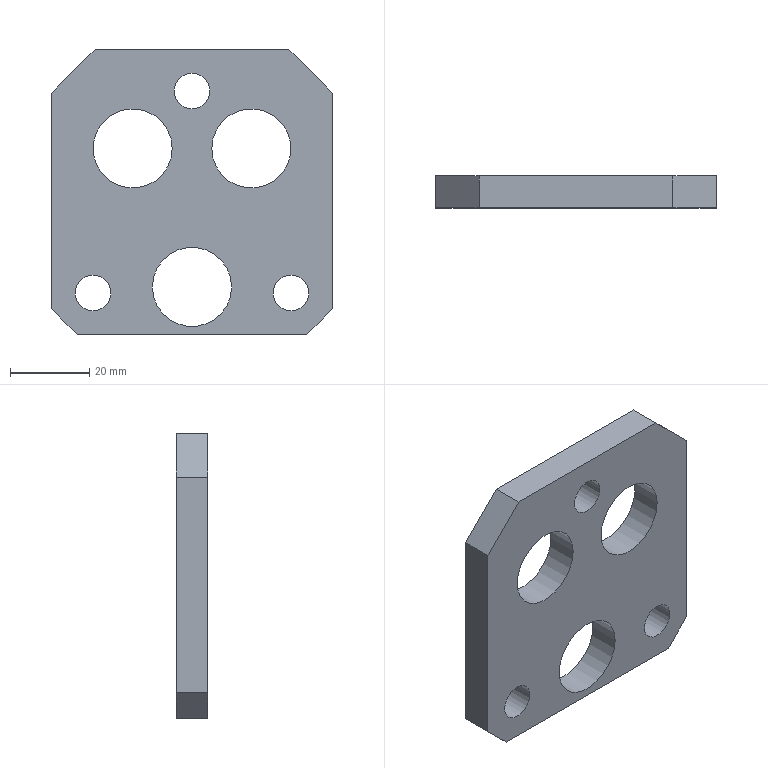Part | STEP file | 1_id610_x_t | 1 solid | 16 faces | box 71 x 8 x 72 mm | volume 30523 mm3 | plane 10 | cylinder 6 | commonest cylinder face diameters 9 x3 20 x3
STEP:
#1=CARTESIAN_POINT('',(0.,0.,0.));
#2=DIRECTION('',(0.,0.,1.));
#3=DIRECTION('',(1.,0.,0.));
#4=AXIS2_PLACEMENT_3D('',#1,#2,#3);
#5=CARTESIAN_POINT('',(720.425,281.527,-85.684));
#6=VERTEX_POINT('',#5);
#7=CARTESIAN_POINT('',(724.925,281.527,-85.684));
#8=DIRECTION('',(0.,1.,0.));
#9=DIRECTION('',(-1.,0.,0.));
#10=AXIS2_PLACEMENT_3D('',#7,#8,#9);
#11=CIRCLE('',#10,4.5);
#12=CARTESIAN_POINT('',(724.925,289.527,-85.684));
#13=DIRECTION('',(0.,-1.,0.));
#14=DIRECTION('',(-1.,0.,0.));
#15=AXIS2_PLACEMENT_3D('',#12,#13,#14);
#16=CYLINDRICAL_SURFACE('',#15,4.5);
#17=CARTESIAN_POINT('',(6.283,8.));
#18=DIRECTION('',(-1.,0.));
#19=VECTOR('',#18,1.);
#20=LINE('',#17,#19);
#21=(GEOMETRIC_REPRESENTATION_CONTEXT(2)PARAMETRIC_REPRESENTATION_CONTEXT()REPRESENTATION_CONTEXT('',''));
#22=DEFINITIONAL_REPRESENTATION('',(#20),#21);
#23=PCURVE('',#16,#22);
#24=CARTESIAN_POINT('',(699.125,281.527,-9.148));
#25=DIRECTION('',(0.,1.,0.));
#26=DIRECTION('',(1.,0.,0.));
#27=AXIS2_PLACEMENT_3D('',#24,#25,#26);
#28=PLANE('',#27);
#29=CARTESIAN_POINT('',(25.8,76.536));
#30=DIRECTION('',(-1.,0.));
#31=AXIS2_PLACEMENT_2D('',#29,#30);
#32=CIRCLE('',#31,4.5);
#33=(GEOMETRIC_REPRESENTATION_CONTEXT(2)PARAMETRIC_REPRESENTATION_CONTEXT()REPRESENTATION_CONTEXT('',''));
#34=DEFINITIONAL_REPRESENTATION('',(#32),#33);
#35=PCURVE('',#28,#34);
#36=SURFACE_CURVE('',#11,(#23,#35),.PCURVE_S1.);
#37=EDGE_CURVE('',#6,#6,#36,.T.);
#38=ORIENTED_EDGE('',*,*,#37,.T.);
#39=CARTESIAN_POINT('',(720.425,289.527,-85.684));
#40=VERTEX_POINT('',#39);
#41=CARTESIAN_POINT('',(720.425,289.527,-85.684));
#42=CARTESIAN_POINT('',(720.425,281.527,-85.684));
#43=B_SPLINE_CURVE_WITH_KNOTS('',1,(#41,#42),.UNSPECIFIED.,.F.,.F.,(2,2),(0.,8.),.PIECEWISE_BEZIER_KNOTS.);
#44=CARTESIAN_POINT('',(0.,0.));
#45=DIRECTION('',(0.,1.));
#46=VECTOR('',#45,1.);
#47=LINE('',#44,#46);
#48=(GEOMETRIC_REPRESENTATION_CONTEXT(2)PARAMETRIC_REPRESENTATION_CONTEXT()REPRESENTATION_CONTEXT('',''));
#49=DEFINITIONAL_REPRESENTATION('',(#47),#48);
#50=PCURVE('',#16,#49);
#51=CARTESIAN_POINT('',(6.283,0.));
#52=DIRECTION('',(0.,1.));
#53=VECTOR('',#52,1.);
#54=LINE('',#51,#53);
#55=(GEOMETRIC_REPRESENTATION_CONTEXT(2)PARAMETRIC_REPRESENTATION_CONTEXT()REPRESENTATION_CONTEXT('',''));
#56=DEFINITIONAL_REPRESENTATION('',(#54),#55);
#57=PCURVE('',#16,#56);
#58=SEAM_CURVE('',#43,(#50,#57),.PCURVE_S1.);
#59=EDGE_CURVE('',#40,#6,#58,.T.);
#60=ORIENTED_EDGE('',*,*,#59,.F.);
#61=CARTESIAN_POINT('',(729.425,289.527,-85.684));
#62=VERTEX_POINT('',#61);
#63=CARTESIAN_POINT('',(724.925,289.527,-85.684));
#64=DIRECTION('',(0.,-1.,0.));
#65=DIRECTION('',(1.,0.,0.));
#66=AXIS2_PLACEMENT_3D('',#63,#64,#65);
#67=CIRCLE('',#66,4.5);
#68=CARTESIAN_POINT('',(-3.142,0.));
#69=DIRECTION('',(1.,0.));
#70=VECTOR('',#69,1.);
#71=LINE('',#68,#70);
#72=(GEOMETRIC_REPRESENTATION_CONTEXT(2)PARAMETRIC_REPRESENTATION_CONTEXT()REPRESENTATION_CONTEXT('',''));
#73=DEFINITIONAL_REPRESENTATION('',(#71),#72);
#74=PCURVE('',#16,#73);
#75=CARTESIAN_POINT('',(699.125,289.527,-9.148));
#76=DIRECTION('',(0.,1.,0.));
#77=DIRECTION('',(1.,0.,0.));
#78=AXIS2_PLACEMENT_3D('',#75,#76,#77);
#79=PLANE('',#78);
#80=CARTESIAN_POINT('',(30.3,76.536));
#81=CARTESIAN_POINT('',(30.3,68.742));
#82=CARTESIAN_POINT('',(23.55,72.639));
#83=CARTESIAN_POINT('',(16.8,76.536));
#84=CARTESIAN_POINT('',(23.55,80.433));
#85=CARTESIAN_POINT('',(30.3,84.33));
#86=CARTESIAN_POINT('',(30.3,76.536));
#87=(BOUNDED_CURVE()B_SPLINE_CURVE(2,(#80,#81,#82,#83,#84,#85,#86),.UNSPECIFIED.,.T.,.F.)B_SPLINE_CURVE_WITH_KNOTS((1,2,2,2,2,1),(-2.094,0.,2.094,4.189,6.283,8.378),.UNSPECIFIED.)CURVE()GEOMETRIC_REPRESENTATION_ITEM()RATIONAL_B_SPLINE_CURVE((1.,0.5,1.,0.5,1.,0.5,1.))REPRESENTATION_ITEM(''));
#88=(GEOMETRIC_REPRESENTATION_CONTEXT(2)PARAMETRIC_REPRESENTATION_CONTEXT()REPRESENTATION_CONTEXT('',''));
#89=DEFINITIONAL_REPRESENTATION('',(#87),#88);
#90=PCURVE('',#79,#89);
#91=SURFACE_CURVE('',#67,(#74,#90),.PCURVE_S1.);
#92=EDGE_CURVE('',#40,#62,#91,.T.);
#93=ORIENTED_EDGE('',*,*,#92,.T.);
#94=CARTESIAN_POINT('',(724.925,289.527,-85.684));
#95=DIRECTION('',(0.,-1.,0.));
#96=DIRECTION('',(1.,0.,0.));
#97=AXIS2_PLACEMENT_3D('',#94,#95,#96);
#98=CIRCLE('',#97,4.5);
#99=CARTESIAN_POINT('',(3.142,0.));
#100=DIRECTION('',(1.,0.));
#101=VECTOR('',#100,1.);
#102=LINE('',#99,#101);
#103=(GEOMETRIC_REPRESENTATION_CONTEXT(2)PARAMETRIC_REPRESENTATION_CONTEXT()REPRESENTATION_CONTEXT('',''));
#104=DEFINITIONAL_REPRESENTATION('',(#102),#103);
#105=PCURVE('',#16,#104);
#106=CARTESIAN_POINT('',(30.3,76.536));
#107=CARTESIAN_POINT('',(30.3,68.742));
#108=CARTESIAN_POINT('',(23.55,72.639));
#109=CARTESIAN_POINT('',(16.8,76.536));
#110=CARTESIAN_POINT('',(23.55,80.433));
#111=CARTESIAN_POINT('',(30.3,84.33));
#112=CARTESIAN_POINT('',(30.3,76.536));
#113=(BOUNDED_CURVE()B_SPLINE_CURVE(2,(#106,#107,#108,#109,#110,#111,#112),.UNSPECIFIED.,.T.,.F.)B_SPLINE_CURVE_WITH_KNOTS((1,2,2,2,2,1),(-2.094,0.,2.094,4.189,6.283,8.378),.UNSPECIFIED.)CURVE()GEOMETRIC_REPRESENTATION_ITEM()RATIONAL_B_SPLINE_CURVE((1.,0.5,1.,0.5,1.,0.5,1.))REPRESENTATION_ITEM(''));
#114=(GEOMETRIC_REPRESENTATION_CONTEXT(2)PARAMETRIC_REPRESENTATION_CONTEXT()REPRESENTATION_CONTEXT('',''));
#115=DEFINITIONAL_REPRESENTATION('',(#113),#114);
#116=PCURVE('',#79,#115);
#117=SURFACE_CURVE('',#98,(#105,#116),.PCURVE_S1.);
#118=EDGE_CURVE('',#62,#40,#117,.T.);
#119=ORIENTED_EDGE('',*,*,#118,.T.);
#120=ORIENTED_EDGE('',*,*,#59,.T.);
#121=EDGE_LOOP('',(#38,#60,#93,#119,#120));
#122=FACE_BOUND('',#121,.F.);
#123=ADVANCED_FACE('',(#122),#16,.F.);
#124=CARTESIAN_POINT('',(774.425,289.527,-24.184));
#125=VERTEX_POINT('',#124);
#126=CARTESIAN_POINT('',(785.425,289.527,-35.184));
#127=VERTEX_POINT('',#126);
#128=CARTESIAN_POINT('',(774.425,289.527,-24.184));
#129=DIRECTION('',(0.7071,0.,-0.7071));
#130=VECTOR('',#129,1.);
#131=LINE('',#128,#130);
#132=CARTESIAN_POINT('',(75.3,15.036));
#133=DIRECTION('',(0.7071,0.7071));
#134=VECTOR('',#133,1.);
#135=LINE('',#132,#134);
#136=(GEOMETRIC_REPRESENTATION_CONTEXT(2)PARAMETRIC_REPRESENTATION_CONTEXT()REPRESENTATION_CONTEXT('',''));
#137=DEFINITIONAL_REPRESENTATION('',(#135),#136);
#138=PCURVE('',#79,#137);
#139=CARTESIAN_POINT('',(729.257,289.527,20.984));
#140=DIRECTION('',(-0.7071,0.,-0.7071));
#141=DIRECTION('',(-0.7071,0.,0.7071));
#142=AXIS2_PLACEMENT_3D('',#139,#140,#141);
#143=PLANE('',#142);
#144=CARTESIAN_POINT('',(-63.877,0.));
#145=DIRECTION('',(-1.,0.));
#146=VECTOR('',#145,1.);
#147=LINE('',#144,#146);
#148=(GEOMETRIC_REPRESENTATION_CONTEXT(2)PARAMETRIC_REPRESENTATION_CONTEXT()REPRESENTATION_CONTEXT('',''));
#149=DEFINITIONAL_REPRESENTATION('',(#147),#148);
#150=PCURVE('',#143,#149);
#151=SURFACE_CURVE('',#131,(#138,#150),.PCURVE_S1.);
#152=EDGE_CURVE('',#125,#127,#151,.T.);
#153=ORIENTED_EDGE('',*,*,#152,.T.);
#154=CARTESIAN_POINT('',(785.425,289.527,-89.684));
#155=VERTEX_POINT('',#154);
#156=CARTESIAN_POINT('',(785.425,289.527,-35.184));
#157=DIRECTION('',(0.,0.,-1.));
#158=VECTOR('',#157,1.);
#159=LINE('',#156,#158);
#160=CARTESIAN_POINT('',(86.3,26.036));
#161=DIRECTION('',(0.,1.));
#162=VECTOR('',#161,1.);
#163=LINE('',#160,#162);
#164=(GEOMETRIC_REPRESENTATION_CONTEXT(2)PARAMETRIC_REPRESENTATION_CONTEXT()REPRESENTATION_CONTEXT('',''));
#165=DEFINITIONAL_REPRESENTATION('',(#163),#164);
#166=PCURVE('',#79,#165);
#167=CARTESIAN_POINT('',(785.425,289.527,159.705));
#168=DIRECTION('',(-1.,0.,0.));
#169=DIRECTION('',(0.,1.,0.));
#170=AXIS2_PLACEMENT_3D('',#167,#168,#169);
#171=PLANE('',#170);
#172=CARTESIAN_POINT('',(0.,194.889));
#173=DIRECTION('',(0.,1.));
#174=VECTOR('',#173,1.);
#175=LINE('',#172,#174);
#176=(GEOMETRIC_REPRESENTATION_CONTEXT(2)PARAMETRIC_REPRESENTATION_CONTEXT()REPRESENTATION_CONTEXT('',''));
#177=DEFINITIONAL_REPRESENTATION('',(#175),#176);
#178=PCURVE('',#171,#177);
#179=SURFACE_CURVE('',#159,(#166,#178),.PCURVE_S1.);
#180=EDGE_CURVE('',#127,#155,#179,.T.);
#181=ORIENTED_EDGE('',*,*,#180,.T.);
#182=CARTESIAN_POINT('',(778.925,289.527,-96.184));
#183=VERTEX_POINT('',#182);
#184=CARTESIAN_POINT('',(785.425,289.527,-89.684));
#185=DIRECTION('',(-0.7071,0.,-0.7071));
#186=VECTOR('',#185,1.);
#187=LINE('',#184,#186);
#188=CARTESIAN_POINT('',(86.3,80.536));
#189=DIRECTION('',(-0.7071,0.7071));
#190=VECTOR('',#189,1.);
#191=LINE('',#188,#190);
#192=(GEOMETRIC_REPRESENTATION_CONTEXT(2)PARAMETRIC_REPRESENTATION_CONTEXT()REPRESENTATION_CONTEXT('',''));
#193=DEFINITIONAL_REPRESENTATION('',(#191),#192);
#194=PCURVE('',#79,#193);
#195=CARTESIAN_POINT('',(775.043,289.527,-100.066));
#196=DIRECTION('',(-0.7071,0.,0.7071));
#197=DIRECTION('',(0.7071,0.,0.7071));
#198=AXIS2_PLACEMENT_3D('',#195,#196,#197);
#199=PLANE('',#198);
#200=CARTESIAN_POINT('',(14.682,0.));
#201=DIRECTION('',(-1.,0.));
#202=VECTOR('',#201,1.);
#203=LINE('',#200,#202);
#204=(GEOMETRIC_REPRESENTATION_CONTEXT(2)PARAMETRIC_REPRESENTATION_CONTEXT()REPRESENTATION_CONTEXT('',''));
#205=DEFINITIONAL_REPRESENTATION('',(#203),#204);
#206=PCURVE('',#199,#205);
#207=SURFACE_CURVE('',#187,(#194,#206),.PCURVE_S1.);
#208=EDGE_CURVE('',#155,#183,#207,.T.);
#209=ORIENTED_EDGE('',*,*,#208,.T.);
#210=CARTESIAN_POINT('',(720.925,289.527,-96.184));
#211=VERTEX_POINT('',#210);
#212=CARTESIAN_POINT('',(778.925,289.527,-96.184));
#213=DIRECTION('',(-1.,0.,0.));
#214=VECTOR('',#213,1.);
#215=LINE('',#212,#214);
#216=CARTESIAN_POINT('',(79.8,87.036));
#217=DIRECTION('',(-1.,0.));
#218=VECTOR('',#217,1.);
#219=LINE('',#216,#218);
#220=(GEOMETRIC_REPRESENTATION_CONTEXT(2)PARAMETRIC_REPRESENTATION_CONTEXT()REPRESENTATION_CONTEXT('',''));
#221=DEFINITIONAL_REPRESENTATION('',(#219),#220);
#222=PCURVE('',#79,#221);
#223=CARTESIAN_POINT('',(699.125,289.527,-96.184));
#224=DIRECTION('',(0.,0.,1.));
#225=DIRECTION('',(0.,-1.,0.));
#226=AXIS2_PLACEMENT_3D('',#223,#224,#225);
#227=PLANE('',#226);
#228=CARTESIAN_POINT('',(0.,79.8));
#229=DIRECTION('',(0.,-1.));
#230=VECTOR('',#229,1.);
#231=LINE('',#228,#230);
#232=(GEOMETRIC_REPRESENTATION_CONTEXT(2)PARAMETRIC_REPRESENTATION_CONTEXT()REPRESENTATION_CONTEXT('',''));
#233=DEFINITIONAL_REPRESENTATION('',(#231),#232);
#234=PCURVE('',#227,#233);
#235=SURFACE_CURVE('',#215,(#222,#234),.PCURVE_S1.);
#236=EDGE_CURVE('',#183,#211,#235,.T.);
#237=ORIENTED_EDGE('',*,*,#236,.T.);
#238=CARTESIAN_POINT('',(714.425,289.527,-89.684));
#239=VERTEX_POINT('',#238);
#240=CARTESIAN_POINT('',(720.925,289.527,-96.184));
#241=DIRECTION('',(-0.7071,0.,0.7071));
#242=VECTOR('',#241,1.);
#243=LINE('',#240,#242);
#244=CARTESIAN_POINT('',(21.8,87.036));
#245=DIRECTION('',(-0.7071,-0.7071));
#246=VECTOR('',#245,1.);
#247=LINE('',#244,#246);
#248=(GEOMETRIC_REPRESENTATION_CONTEXT(2)PARAMETRIC_REPRESENTATION_CONTEXT()REPRESENTATION_CONTEXT('',''));
#249=DEFINITIONAL_REPRESENTATION('',(#247),#248);
#250=PCURVE('',#79,#249);
#251=CARTESIAN_POINT('',(674.007,289.527,-49.266));
#252=DIRECTION('',(0.7071,0.,0.7071));
#253=DIRECTION('',(0.7071,0.,-0.7071));
#254=AXIS2_PLACEMENT_3D('',#251,#252,#253);
#255=PLANE('',#254);
#256=CARTESIAN_POINT('',(66.352,0.));
#257=DIRECTION('',(-1.,0.));
#258=VECTOR('',#257,1.);
#259=LINE('',#256,#258);
#260=(GEOMETRIC_REPRESENTATION_CONTEXT(2)PARAMETRIC_REPRESENTATION_CONTEXT()REPRESENTATION_CONTEXT('',''));
#261=DEFINITIONAL_REPRESENTATION('',(#259),#260);
#262=PCURVE('',#255,#261);
#263=SURFACE_CURVE('',#243,(#250,#262),.PCURVE_S1.);
#264=EDGE_CURVE('',#211,#239,#263,.T.);
#265=ORIENTED_EDGE('',*,*,#264,.T.);
#266=CARTESIAN_POINT('',(714.425,289.527,-35.184));
#267=VERTEX_POINT('',#266);
#268=CARTESIAN_POINT('',(714.425,289.527,-89.684));
#269=DIRECTION('',(0.,0.,1.));
#270=VECTOR('',#269,1.);
#271=LINE('',#268,#270);
#272=CARTESIAN_POINT('',(15.3,80.536));
#273=DIRECTION('',(0.,-1.));
#274=VECTOR('',#273,1.);
#275=LINE('',#272,#274);
#276=(GEOMETRIC_REPRESENTATION_CONTEXT(2)PARAMETRIC_REPRESENTATION_CONTEXT()REPRESENTATION_CONTEXT('',''));
#277=DEFINITIONAL_REPRESENTATION('',(#275),#276);
#278=PCURVE('',#79,#277);
#279=CARTESIAN_POINT('',(714.425,289.527,-255.215));
#280=DIRECTION('',(1.,0.,0.));
#281=DIRECTION('',(0.,-1.,0.));
#282=AXIS2_PLACEMENT_3D('',#279,#280,#281);
#283=PLANE('',#282);
#284=CARTESIAN_POINT('',(0.,-165.531));
#285=DIRECTION('',(0.,-1.));
#286=VECTOR('',#285,1.);
#287=LINE('',#284,#286);
#288=(GEOMETRIC_REPRESENTATION_CONTEXT(2)PARAMETRIC_REPRESENTATION_CONTEXT()REPRESENTATION_CONTEXT('',''));
#289=DEFINITIONAL_REPRESENTATION('',(#287),#288);
#290=PCURVE('',#283,#289);
#291=SURFACE_CURVE('',#271,(#278,#290),.PCURVE_S1.);
#292=EDGE_CURVE('',#239,#267,#291,.T.);
#293=ORIENTED_EDGE('',*,*,#292,.T.);
#294=CARTESIAN_POINT('',(725.425,289.527,-24.184));
#295=VERTEX_POINT('',#294);
#296=CARTESIAN_POINT('',(714.425,289.527,-35.184));
#297=DIRECTION('',(0.7071,0.,0.7071));
#298=VECTOR('',#297,1.);
#299=LINE('',#296,#298);
#300=CARTESIAN_POINT('',(15.3,26.036));
#301=DIRECTION('',(0.7071,-0.7071));
#302=VECTOR('',#301,1.);
#303=LINE('',#300,#302);
#304=(GEOMETRIC_REPRESENTATION_CONTEXT(2)PARAMETRIC_REPRESENTATION_CONTEXT()REPRESENTATION_CONTEXT('',''));
#305=DEFINITIONAL_REPRESENTATION('',(#303),#304);
#306=PCURVE('',#79,#305);
#307=CARTESIAN_POINT('',(719.793,289.527,-29.816));
#308=DIRECTION('',(0.7071,0.,-0.7071));
#309=DIRECTION('',(-0.7071,0.,-0.7071));
#310=AXIS2_PLACEMENT_3D('',#307,#308,#309);
#311=PLANE('',#310);
#312=CARTESIAN_POINT('',(7.591,0.));
#313=DIRECTION('',(-1.,0.));
#314=VECTOR('',#313,1.);
#315=LINE('',#312,#314);
#316=(GEOMETRIC_REPRESENTATION_CONTEXT(2)PARAMETRIC_REPRESENTATION_CONTEXT()REPRESENTATION_CONTEXT('',''));
#317=DEFINITIONAL_REPRESENTATION('',(#315),#316);
#318=PCURVE('',#311,#317);
#319=SURFACE_CURVE('',#299,(#306,#318),.PCURVE_S1.);
#320=EDGE_CURVE('',#267,#295,#319,.T.);
#321=ORIENTED_EDGE('',*,*,#320,.T.);
#322=CARTESIAN_POINT('',(725.425,289.527,-24.184));
#323=DIRECTION('',(1.,0.,0.));
#324=VECTOR('',#323,1.);
#325=LINE('',#322,#324);
#326=CARTESIAN_POINT('',(26.3,15.036));
#327=DIRECTION('',(1.,0.));
#328=VECTOR('',#327,1.);
#329=LINE('',#326,#328);
#330=(GEOMETRIC_REPRESENTATION_CONTEXT(2)PARAMETRIC_REPRESENTATION_CONTEXT()REPRESENTATION_CONTEXT('',''));
#331=DEFINITIONAL_REPRESENTATION('',(#329),#330);
#332=PCURVE('',#79,#331);
#333=CARTESIAN_POINT('',(699.125,289.527,-24.184));
#334=DIRECTION('',(0.,0.,-1.));
#335=DIRECTION('',(0.,1.,0.));
#336=AXIS2_PLACEMENT_3D('',#333,#334,#335);
#337=PLANE('',#336);
#338=CARTESIAN_POINT('',(0.,26.3));
#339=DIRECTION('',(0.,1.));
#340=VECTOR('',#339,1.);
#341=LINE('',#338,#340);
#342=(GEOMETRIC_REPRESENTATION_CONTEXT(2)PARAMETRIC_REPRESENTATION_CONTEXT()REPRESENTATION_CONTEXT('',''));
#343=DEFINITIONAL_REPRESENTATION('',(#341),#342);
#344=PCURVE('',#337,#343);
#345=SURFACE_CURVE('',#325,(#332,#344),.PCURVE_S1.);
#346=EDGE_CURVE('',#295,#125,#345,.T.);
#347=ORIENTED_EDGE('',*,*,#346,.T.);
#348=EDGE_LOOP('',(#153,#181,#209,#237,#265,#293,#321,#347));
#349=FACE_BOUND('',#348,.T.);
#350=CARTESIAN_POINT('',(774.925,289.527,-49.184));
#351=VERTEX_POINT('',#350);
#352=CARTESIAN_POINT('',(754.925,289.527,-49.184));
#353=VERTEX_POINT('',#352);
#354=CARTESIAN_POINT('',(764.925,289.527,-49.184));
#355=DIRECTION('',(0.,-1.,0.));
#356=DIRECTION('',(1.,0.,0.));
#357=AXIS2_PLACEMENT_3D('',#354,#355,#356);
#358=CIRCLE('',#357,10.);
#359=CARTESIAN_POINT('',(75.8,40.036));
#360=CARTESIAN_POINT('',(75.8,22.715));
#361=CARTESIAN_POINT('',(60.8,31.376));
#362=CARTESIAN_POINT('',(45.8,40.036));
#363=CARTESIAN_POINT('',(60.8,48.696));
#364=CARTESIAN_POINT('',(75.8,57.357));
#365=CARTESIAN_POINT('',(75.8,40.036));
#366=(BOUNDED_CURVE()B_SPLINE_CURVE(2,(#359,#360,#361,#362,#363,#364,#365),.UNSPECIFIED.,.T.,.F.)B_SPLINE_CURVE_WITH_KNOTS((1,2,2,2,2,1),(-2.094,0.,2.094,4.189,6.283,8.378),.UNSPECIFIED.)CURVE()GEOMETRIC_REPRESENTATION_ITEM()RATIONAL_B_SPLINE_CURVE((1.,0.5,1.,0.5,1.,0.5,1.))REPRESENTATION_ITEM(''));
#367=(GEOMETRIC_REPRESENTATION_CONTEXT(2)PARAMETRIC_REPRESENTATION_CONTEXT()REPRESENTATION_CONTEXT('',''));
#368=DEFINITIONAL_REPRESENTATION('',(#366),#367);
#369=PCURVE('',#79,#368);
#370=CARTESIAN_POINT('',(764.925,289.527,-49.184));
#371=DIRECTION('',(0.,-1.,0.));
#372=DIRECTION('',(-1.,0.,0.));
#373=AXIS2_PLACEMENT_3D('',#370,#371,#372);
#374=CYLINDRICAL_SURFACE('',#373,10.);
#375=CARTESIAN_POINT('',(3.142,0.));
#376=DIRECTION('',(1.,0.));
#377=VECTOR('',#376,1.);
#378=LINE('',#375,#377);
#379=(GEOMETRIC_REPRESENTATION_CONTEXT(2)PARAMETRIC_REPRESENTATION_CONTEXT()REPRESENTATION_CONTEXT('',''));
#380=DEFINITIONAL_REPRESENTATION('',(#378),#379);
#381=PCURVE('',#374,#380);
#382=SURFACE_CURVE('',#358,(#369,#381),.PCURVE_S1.);
#383=EDGE_CURVE('',#351,#353,#382,.T.);
#384=ORIENTED_EDGE('',*,*,#383,.T.);
#385=CARTESIAN_POINT('',(764.925,289.527,-49.184));
#386=DIRECTION('',(0.,-1.,0.));
#387=DIRECTION('',(1.,0.,0.));
#388=AXIS2_PLACEMENT_3D('',#385,#386,#387);
#389=CIRCLE('',#388,10.);
#390=CARTESIAN_POINT('',(75.8,40.036));
#391=CARTESIAN_POINT('',(75.8,22.715));
#392=CARTESIAN_POINT('',(60.8,31.376));
#393=CARTESIAN_POINT('',(45.8,40.036));
#394=CARTESIAN_POINT('',(60.8,48.696));
#395=CARTESIAN_POINT('',(75.8,57.357));
#396=CARTESIAN_POINT('',(75.8,40.036));
#397=(BOUNDED_CURVE()B_SPLINE_CURVE(2,(#390,#391,#392,#393,#394,#395,#396),.UNSPECIFIED.,.T.,.F.)B_SPLINE_CURVE_WITH_KNOTS((1,2,2,2,2,1),(-2.094,0.,2.094,4.189,6.283,8.378),.UNSPECIFIED.)CURVE()GEOMETRIC_REPRESENTATION_ITEM()RATIONAL_B_SPLINE_CURVE((1.,0.5,1.,0.5,1.,0.5,1.))REPRESENTATION_ITEM(''));
#398=(GEOMETRIC_REPRESENTATION_CONTEXT(2)PARAMETRIC_REPRESENTATION_CONTEXT()REPRESENTATION_CONTEXT('',''));
#399=DEFINITIONAL_REPRESENTATION('',(#397),#398);
#400=PCURVE('',#79,#399);
#401=CARTESIAN_POINT('',(-3.142,0.));
#402=DIRECTION('',(1.,0.));
#403=VECTOR('',#402,1.);
#404=LINE('',#401,#403);
#405=(GEOMETRIC_REPRESENTATION_CONTEXT(2)PARAMETRIC_REPRESENTATION_CONTEXT()REPRESENTATION_CONTEXT('',''));
#406=DEFINITIONAL_REPRESENTATION('',(#404),#405);
#407=PCURVE('',#374,#406);
#408=SURFACE_CURVE('',#389,(#400,#407),.PCURVE_S1.);
#409=EDGE_CURVE('',#353,#351,#408,.T.);
#410=ORIENTED_EDGE('',*,*,#409,.T.);
#411=EDGE_LOOP('',(#384,#410));
#412=FACE_BOUND('',#411,.T.);
#413=CARTESIAN_POINT('',(759.925,289.527,-84.184));
#414=VERTEX_POINT('',#413);
#415=CARTESIAN_POINT('',(749.925,289.527,-84.184));
#416=DIRECTION('',(0.,-1.,0.));
#417=DIRECTION('',(1.,0.,0.));
#418=AXIS2_PLACEMENT_3D('',#415,#416,#417);
#419=CIRCLE('',#418,10.);
#420=CARTESIAN_POINT('',(60.8,75.036));
#421=CARTESIAN_POINT('',(60.8,57.715));
#422=CARTESIAN_POINT('',(45.8,66.376));
#423=CARTESIAN_POINT('',(30.8,75.036));
#424=CARTESIAN_POINT('',(45.8,83.696));
#425=CARTESIAN_POINT('',(60.8,92.357));
#426=CARTESIAN_POINT('',(60.8,75.036));
#427=(BOUNDED_CURVE()B_SPLINE_CURVE(2,(#420,#421,#422,#423,#424,#425,#426),.UNSPECIFIED.,.T.,.F.)B_SPLINE_CURVE_WITH_KNOTS((1,2,2,2,2,1),(-2.094,0.,2.094,4.189,6.283,8.378),.UNSPECIFIED.)CURVE()GEOMETRIC_REPRESENTATION_ITEM()RATIONAL_B_SPLINE_CURVE((1.,0.5,1.,0.5,1.,0.5,1.))REPRESENTATION_ITEM(''));
#428=(GEOMETRIC_REPRESENTATION_CONTEXT(2)PARAMETRIC_REPRESENTATION_CONTEXT()REPRESENTATION_CONTEXT('',''));
#429=DEFINITIONAL_REPRESENTATION('',(#427),#428);
#430=PCURVE('',#79,#429);
#431=CARTESIAN_POINT('',(749.925,289.527,-84.184));
#432=DIRECTION('',(0.,-1.,0.));
#433=DIRECTION('',(-1.,0.,0.));
#434=AXIS2_PLACEMENT_3D('',#431,#432,#433);
#435=CYLINDRICAL_SURFACE('',#434,10.);
#436=CARTESIAN_POINT('',(3.142,0.));
#437=DIRECTION('',(1.,0.));
#438=VECTOR('',#437,1.);
#439=LINE('',#436,#438);
#440=(GEOMETRIC_REPRESENTATION_CONTEXT(2)PARAMETRIC_REPRESENTATION_CONTEXT()REPRESENTATION_CONTEXT('',''));
#441=DEFINITIONAL_REPRESENTATION('',(#439),#440);
#442=PCURVE('',#435,#441);
#443=SURFACE_CURVE('',#419,(#430,#442),.PCURVE_S1.);
#444=EDGE_CURVE('',#414,#414,#443,.T.);
#445=ORIENTED_EDGE('',*,*,#444,.T.);
#446=EDGE_LOOP('',(#445));
#447=FACE_BOUND('',#446,.T.);
#448=CARTESIAN_POINT('',(744.925,289.527,-49.184));
#449=VERTEX_POINT('',#448);
#450=CARTESIAN_POINT('',(734.925,289.527,-49.184));
#451=DIRECTION('',(0.,-1.,0.));
#452=DIRECTION('',(1.,0.,0.));
#453=AXIS2_PLACEMENT_3D('',#450,#451,#452);
#454=CIRCLE('',#453,10.);
#455=CARTESIAN_POINT('',(45.8,40.036));
#456=CARTESIAN_POINT('',(45.8,22.715));
#457=CARTESIAN_POINT('',(30.8,31.376));
#458=CARTESIAN_POINT('',(15.8,40.036));
#459=CARTESIAN_POINT('',(30.8,48.696));
#460=CARTESIAN_POINT('',(45.8,57.357));
#461=CARTESIAN_POINT('',(45.8,40.036));
#462=(BOUNDED_CURVE()B_SPLINE_CURVE(2,(#455,#456,#457,#458,#459,#460,#461),.UNSPECIFIED.,.T.,.F.)B_SPLINE_CURVE_WITH_KNOTS((1,2,2,2,2,1),(-2.094,0.,2.094,4.189,6.283,8.378),.UNSPECIFIED.)CURVE()GEOMETRIC_REPRESENTATION_ITEM()RATIONAL_B_SPLINE_CURVE((1.,0.5,1.,0.5,1.,0.5,1.))REPRESENTATION_ITEM(''));
#463=(GEOMETRIC_REPRESENTATION_CONTEXT(2)PARAMETRIC_REPRESENTATION_CONTEXT()REPRESENTATION_CONTEXT('',''));
#464=DEFINITIONAL_REPRESENTATION('',(#462),#463);
#465=PCURVE('',#79,#464);
#466=CARTESIAN_POINT('',(734.925,289.527,-49.184));
#467=DIRECTION('',(0.,-1.,0.));
#468=DIRECTION('',(-1.,0.,0.));
#469=AXIS2_PLACEMENT_3D('',#466,#467,#468);
#470=CYLINDRICAL_SURFACE('',#469,10.);
#471=CARTESIAN_POINT('',(3.142,0.));
#472=DIRECTION('',(1.,0.));
#473=VECTOR('',#472,1.);
#474=LINE('',#471,#473);
#475=(GEOMETRIC_REPRESENTATION_CONTEXT(2)PARAMETRIC_REPRESENTATION_CONTEXT()REPRESENTATION_CONTEXT('',''));
#476=DEFINITIONAL_REPRESENTATION('',(#474),#475);
#477=PCURVE('',#470,#476);
#478=SURFACE_CURVE('',#454,(#465,#477),.PCURVE_S1.);
#479=EDGE_CURVE('',#449,#449,#478,.T.);
#480=ORIENTED_EDGE('',*,*,#479,.T.);
#481=EDGE_LOOP('',(#480));
#482=FACE_BOUND('',#481,.T.);
#483=CARTESIAN_POINT('',(745.425,289.527,-34.684));
#484=VERTEX_POINT('',#483);
#485=CARTESIAN_POINT('',(749.925,289.527,-34.684));
#486=DIRECTION('',(0.,-1.,0.));
#487=DIRECTION('',(-1.,0.,0.));
#488=AXIS2_PLACEMENT_3D('',#485,#486,#487);
#489=CIRCLE('',#488,4.5);
#490=CARTESIAN_POINT('',(46.3,25.536));
#491=CARTESIAN_POINT('',(46.3,33.33));
#492=CARTESIAN_POINT('',(53.05,29.433));
#493=CARTESIAN_POINT('',(59.8,25.536));
#494=CARTESIAN_POINT('',(53.05,21.639));
#495=CARTESIAN_POINT('',(46.3,17.742));
#496=CARTESIAN_POINT('',(46.3,25.536));
#497=(BOUNDED_CURVE()B_SPLINE_CURVE(2,(#490,#491,#492,#493,#494,#495,#496),.UNSPECIFIED.,.T.,.F.)B_SPLINE_CURVE_WITH_KNOTS((1,2,2,2,2,1),(-2.094,0.,2.094,4.189,6.283,8.378),.UNSPECIFIED.)CURVE()GEOMETRIC_REPRESENTATION_ITEM()RATIONAL_B_SPLINE_CURVE((1.,0.5,1.,0.5,1.,0.5,1.))REPRESENTATION_ITEM(''));
#498=(GEOMETRIC_REPRESENTATION_CONTEXT(2)PARAMETRIC_REPRESENTATION_CONTEXT()REPRESENTATION_CONTEXT('',''));
#499=DEFINITIONAL_REPRESENTATION('',(#497),#498);
#500=PCURVE('',#79,#499);
#501=CARTESIAN_POINT('',(749.925,289.527,-34.684));
#502=DIRECTION('',(0.,-1.,0.));
#503=DIRECTION('',(-1.,0.,0.));
#504=AXIS2_PLACEMENT_3D('',#501,#502,#503);
#505=CYLINDRICAL_SURFACE('',#504,4.5);
#506=CARTESIAN_POINT('',(0.,0.));
#507=DIRECTION('',(1.,0.));
#508=VECTOR('',#507,1.);
#509=LINE('',#506,#508);
#510=(GEOMETRIC_REPRESENTATION_CONTEXT(2)PARAMETRIC_REPRESENTATION_CONTEXT()REPRESENTATION_CONTEXT('',''));
#511=DEFINITIONAL_REPRESENTATION('',(#509),#510);
#512=PCURVE('',#505,#511);
#513=SURFACE_CURVE('',#489,(#500,#512),.PCURVE_S1.);
#514=EDGE_CURVE('',#484,#484,#513,.T.);
#515=ORIENTED_EDGE('',*,*,#514,.T.);
#516=EDGE_LOOP('',(#515));
#517=FACE_BOUND('',#516,.T.);
#518=ORIENTED_EDGE('',*,*,#118,.T.);
#519=ORIENTED_EDGE('',*,*,#92,.T.);
#520=EDGE_LOOP('',(#518,#519));
#521=FACE_BOUND('',#520,.T.);
#522=CARTESIAN_POINT('',(779.425,289.527,-85.684));
#523=VERTEX_POINT('',#522);
#524=CARTESIAN_POINT('',(774.925,289.527,-85.684));
#525=DIRECTION('',(0.,-1.,0.));
#526=DIRECTION('',(1.,0.,0.));
#527=AXIS2_PLACEMENT_3D('',#524,#525,#526);
#528=CIRCLE('',#527,4.5);
#529=CARTESIAN_POINT('',(80.3,76.536));
#530=CARTESIAN_POINT('',(80.3,68.742));
#531=CARTESIAN_POINT('',(73.55,72.639));
#532=CARTESIAN_POINT('',(66.8,76.536));
#533=CARTESIAN_POINT('',(73.55,80.433));
#534=CARTESIAN_POINT('',(80.3,84.33));
#535=CARTESIAN_POINT('',(80.3,76.536));
#536=(BOUNDED_CURVE()B_SPLINE_CURVE(2,(#529,#530,#531,#532,#533,#534,#535),.UNSPECIFIED.,.T.,.F.)B_SPLINE_CURVE_WITH_KNOTS((1,2,2,2,2,1),(-2.094,0.,2.094,4.189,6.283,8.378),.UNSPECIFIED.)CURVE()GEOMETRIC_REPRESENTATION_ITEM()RATIONAL_B_SPLINE_CURVE((1.,0.5,1.,0.5,1.,0.5,1.))REPRESENTATION_ITEM(''));
#537=(GEOMETRIC_REPRESENTATION_CONTEXT(2)PARAMETRIC_REPRESENTATION_CONTEXT()REPRESENTATION_CONTEXT('',''));
#538=DEFINITIONAL_REPRESENTATION('',(#536),#537);
#539=PCURVE('',#79,#538);
#540=CARTESIAN_POINT('',(774.925,289.527,-85.684));
#541=DIRECTION('',(0.,-1.,0.));
#542=DIRECTION('',(-1.,0.,0.));
#543=AXIS2_PLACEMENT_3D('',#540,#541,#542);
#544=CYLINDRICAL_SURFACE('',#543,4.5);
#545=CARTESIAN_POINT('',(3.142,0.));
#546=DIRECTION('',(1.,0.));
#547=VECTOR('',#546,1.);
#548=LINE('',#545,#547);
#549=(GEOMETRIC_REPRESENTATION_CONTEXT(2)PARAMETRIC_REPRESENTATION_CONTEXT()REPRESENTATION_CONTEXT('',''));
#550=DEFINITIONAL_REPRESENTATION('',(#548),#549);
#551=PCURVE('',#544,#550);
#552=SURFACE_CURVE('',#528,(#539,#551),.PCURVE_S1.);
#553=EDGE_CURVE('',#523,#523,#552,.T.);
#554=ORIENTED_EDGE('',*,*,#553,.T.);
#555=EDGE_LOOP('',(#554));
#556=FACE_BOUND('',#555,.T.);
#557=ADVANCED_FACE('',(#349,#412,#447,#482,#517,#521,#556),#79,.T.);
#558=CARTESIAN_POINT('',(754.925,281.527,-49.184));
#559=VERTEX_POINT('',#558);
#560=CARTESIAN_POINT('',(764.925,281.527,-49.184));
#561=DIRECTION('',(0.,1.,0.));
#562=DIRECTION('',(-1.,0.,0.));
#563=AXIS2_PLACEMENT_3D('',#560,#561,#562);
#564=CIRCLE('',#563,10.);
#565=CARTESIAN_POINT('',(6.283,8.));
#566=DIRECTION('',(-1.,0.));
#567=VECTOR('',#566,1.);
#568=LINE('',#565,#567);
#569=(GEOMETRIC_REPRESENTATION_CONTEXT(2)PARAMETRIC_REPRESENTATION_CONTEXT()REPRESENTATION_CONTEXT('',''));
#570=DEFINITIONAL_REPRESENTATION('',(#568),#569);
#571=PCURVE('',#374,#570);
#572=CARTESIAN_POINT('',(65.8,40.036));
#573=DIRECTION('',(-1.,0.));
#574=AXIS2_PLACEMENT_2D('',#572,#573);
#575=CIRCLE('',#574,10.);
#576=(GEOMETRIC_REPRESENTATION_CONTEXT(2)PARAMETRIC_REPRESENTATION_CONTEXT()REPRESENTATION_CONTEXT('',''));
#577=DEFINITIONAL_REPRESENTATION('',(#575),#576);
#578=PCURVE('',#28,#577);
#579=SURFACE_CURVE('',#564,(#571,#578),.PCURVE_S1.);
#580=EDGE_CURVE('',#559,#559,#579,.T.);
#581=ORIENTED_EDGE('',*,*,#580,.T.);
#582=CARTESIAN_POINT('',(754.925,289.527,-49.184));
#583=CARTESIAN_POINT('',(754.925,281.527,-49.184));
#584=B_SPLINE_CURVE_WITH_KNOTS('',1,(#582,#583),.UNSPECIFIED.,.F.,.F.,(2,2),(0.,8.),.PIECEWISE_BEZIER_KNOTS.);
#585=CARTESIAN_POINT('',(0.,0.));
#586=DIRECTION('',(0.,1.));
#587=VECTOR('',#586,1.);
#588=LINE('',#585,#587);
#589=(GEOMETRIC_REPRESENTATION_CONTEXT(2)PARAMETRIC_REPRESENTATION_CONTEXT()REPRESENTATION_CONTEXT('',''));
#590=DEFINITIONAL_REPRESENTATION('',(#588),#589);
#591=PCURVE('',#374,#590);
#592=CARTESIAN_POINT('',(6.283,0.));
#593=DIRECTION('',(0.,1.));
#594=VECTOR('',#593,1.);
#595=LINE('',#592,#594);
#596=(GEOMETRIC_REPRESENTATION_CONTEXT(2)PARAMETRIC_REPRESENTATION_CONTEXT()REPRESENTATION_CONTEXT('',''));
#597=DEFINITIONAL_REPRESENTATION('',(#595),#596);
#598=PCURVE('',#374,#597);
#599=SEAM_CURVE('',#584,(#591,#598),.PCURVE_S1.);
#600=EDGE_CURVE('',#353,#559,#599,.T.);
#601=ORIENTED_EDGE('',*,*,#600,.F.);
#602=ORIENTED_EDGE('',*,*,#409,.T.);
#603=ORIENTED_EDGE('',*,*,#383,.T.);
#604=ORIENTED_EDGE('',*,*,#600,.T.);
#605=EDGE_LOOP('',(#581,#601,#602,#603,#604));
#606=FACE_BOUND('',#605,.F.);
#607=ADVANCED_FACE('',(#606),#374,.F.);
#608=CARTESIAN_POINT('',(725.425,281.527,-24.184));
#609=VERTEX_POINT('',#608);
#610=CARTESIAN_POINT('',(714.425,281.527,-35.184));
#611=VERTEX_POINT('',#610);
#612=CARTESIAN_POINT('',(725.425,281.527,-24.184));
#613=DIRECTION('',(-0.7071,0.,-0.7071));
#614=VECTOR('',#613,1.);
#615=LINE('',#612,#614);
#616=CARTESIAN_POINT('',(26.3,15.036));
#617=DIRECTION('',(-0.7071,0.7071));
#618=VECTOR('',#617,1.);
#619=LINE('',#616,#618);
#620=(GEOMETRIC_REPRESENTATION_CONTEXT(2)PARAMETRIC_REPRESENTATION_CONTEXT()REPRESENTATION_CONTEXT('',''));
#621=DEFINITIONAL_REPRESENTATION('',(#619),#620);
#622=PCURVE('',#28,#621);
#623=CARTESIAN_POINT('',(-7.965,-8.));
#624=DIRECTION('',(1.,0.));
#625=VECTOR('',#624,1.);
#626=LINE('',#623,#625);
#627=(GEOMETRIC_REPRESENTATION_CONTEXT(2)PARAMETRIC_REPRESENTATION_CONTEXT()REPRESENTATION_CONTEXT('',''));
#628=DEFINITIONAL_REPRESENTATION('',(#626),#627);
#629=PCURVE('',#311,#628);
#630=SURFACE_CURVE('',#615,(#622,#629),.PCURVE_S1.);
#631=EDGE_CURVE('',#609,#611,#630,.T.);
#632=ORIENTED_EDGE('',*,*,#631,.T.);
#633=CARTESIAN_POINT('',(714.425,281.527,-89.684));
#634=VERTEX_POINT('',#633);
#635=CARTESIAN_POINT('',(714.425,281.527,-89.684));
#636=DIRECTION('',(0.,0.,1.));
#637=VECTOR('',#636,1.);
#638=LINE('',#635,#637);
#639=CARTESIAN_POINT('',(15.3,80.536));
#640=DIRECTION('',(0.,-1.));
#641=VECTOR('',#640,1.);
#642=LINE('',#639,#641);
#643=(GEOMETRIC_REPRESENTATION_CONTEXT(2)PARAMETRIC_REPRESENTATION_CONTEXT()REPRESENTATION_CONTEXT('',''));
#644=DEFINITIONAL_REPRESENTATION('',(#642),#643);
#645=PCURVE('',#28,#644);
#646=CARTESIAN_POINT('',(8.,-165.531));
#647=DIRECTION('',(0.,-1.));
#648=VECTOR('',#647,1.);
#649=LINE('',#646,#648);
#650=(GEOMETRIC_REPRESENTATION_CONTEXT(2)PARAMETRIC_REPRESENTATION_CONTEXT()REPRESENTATION_CONTEXT('',''));
#651=DEFINITIONAL_REPRESENTATION('',(#649),#650);
#652=PCURVE('',#283,#651);
#653=SURFACE_CURVE('',#638,(#645,#652),.PCURVE_S1.);
#654=EDGE_CURVE('',#634,#611,#653,.T.);
#655=ORIENTED_EDGE('',*,*,#654,.F.);
#656=CARTESIAN_POINT('',(720.925,281.527,-96.184));
#657=VERTEX_POINT('',#656);
#658=CARTESIAN_POINT('',(714.425,281.527,-89.684));
#659=DIRECTION('',(0.7071,0.,-0.7071));
#660=VECTOR('',#659,1.);
#661=LINE('',#658,#660);
#662=CARTESIAN_POINT('',(15.3,80.536));
#663=DIRECTION('',(0.7071,0.7071));
#664=VECTOR('',#663,1.);
#665=LINE('',#662,#664);
#666=(GEOMETRIC_REPRESENTATION_CONTEXT(2)PARAMETRIC_REPRESENTATION_CONTEXT()REPRESENTATION_CONTEXT('',''));
#667=DEFINITIONAL_REPRESENTATION('',(#665),#666);
#668=PCURVE('',#28,#667);
#669=CARTESIAN_POINT('',(57.16,-8.));
#670=DIRECTION('',(1.,0.));
#671=VECTOR('',#670,1.);
#672=LINE('',#669,#671);
#673=(GEOMETRIC_REPRESENTATION_CONTEXT(2)PARAMETRIC_REPRESENTATION_CONTEXT()REPRESENTATION_CONTEXT('',''));
#674=DEFINITIONAL_REPRESENTATION('',(#672),#673);
#675=PCURVE('',#255,#674);
#676=SURFACE_CURVE('',#661,(#668,#675),.PCURVE_S1.);
#677=EDGE_CURVE('',#634,#657,#676,.T.);
#678=ORIENTED_EDGE('',*,*,#677,.T.);
#679=CARTESIAN_POINT('',(778.925,281.527,-96.184));
#680=VERTEX_POINT('',#679);
#681=CARTESIAN_POINT('',(778.925,281.527,-96.184));
#682=DIRECTION('',(-1.,0.,0.));
#683=VECTOR('',#682,1.);
#684=LINE('',#681,#683);
#685=CARTESIAN_POINT('',(79.8,87.036));
#686=DIRECTION('',(-1.,0.));
#687=VECTOR('',#686,1.);
#688=LINE('',#685,#687);
#689=(GEOMETRIC_REPRESENTATION_CONTEXT(2)PARAMETRIC_REPRESENTATION_CONTEXT()REPRESENTATION_CONTEXT('',''));
#690=DEFINITIONAL_REPRESENTATION('',(#688),#689);
#691=PCURVE('',#28,#690);
#692=CARTESIAN_POINT('',(8.,79.8));
#693=DIRECTION('',(0.,-1.));
#694=VECTOR('',#693,1.);
#695=LINE('',#692,#694);
#696=(GEOMETRIC_REPRESENTATION_CONTEXT(2)PARAMETRIC_REPRESENTATION_CONTEXT()REPRESENTATION_CONTEXT('',''));
#697=DEFINITIONAL_REPRESENTATION('',(#695),#696);
#698=PCURVE('',#227,#697);
#699=SURFACE_CURVE('',#684,(#691,#698),.PCURVE_S1.);
#700=EDGE_CURVE('',#680,#657,#699,.T.);
#701=ORIENTED_EDGE('',*,*,#700,.F.);
#702=CARTESIAN_POINT('',(785.425,281.527,-89.684));
#703=VERTEX_POINT('',#702);
#704=CARTESIAN_POINT('',(778.925,281.527,-96.184));
#705=DIRECTION('',(0.7071,0.,0.7071));
#706=VECTOR('',#705,1.);
#707=LINE('',#704,#706);
#708=CARTESIAN_POINT('',(79.8,87.036));
#709=DIRECTION('',(0.7071,-0.7071));
#710=VECTOR('',#709,1.);
#711=LINE('',#708,#710);
#712=(GEOMETRIC_REPRESENTATION_CONTEXT(2)PARAMETRIC_REPRESENTATION_CONTEXT()REPRESENTATION_CONTEXT('',''));
#713=DEFINITIONAL_REPRESENTATION('',(#711),#712);
#714=PCURVE('',#28,#713);
#715=CARTESIAN_POINT('',(5.49,-8.));
#716=DIRECTION('',(1.,0.));
#717=VECTOR('',#716,1.);
#718=LINE('',#715,#717);
#719=(GEOMETRIC_REPRESENTATION_CONTEXT(2)PARAMETRIC_REPRESENTATION_CONTEXT()REPRESENTATION_CONTEXT('',''));
#720=DEFINITIONAL_REPRESENTATION('',(#718),#719);
#721=PCURVE('',#199,#720);
#722=SURFACE_CURVE('',#707,(#714,#721),.PCURVE_S1.);
#723=EDGE_CURVE('',#680,#703,#722,.T.);
#724=ORIENTED_EDGE('',*,*,#723,.T.);
#725=CARTESIAN_POINT('',(785.425,281.527,-35.184));
#726=VERTEX_POINT('',#725);
#727=CARTESIAN_POINT('',(785.425,281.527,-35.184));
#728=DIRECTION('',(0.,0.,-1.));
#729=VECTOR('',#728,1.);
#730=LINE('',#727,#729);
#731=CARTESIAN_POINT('',(86.3,26.036));
#732=DIRECTION('',(0.,1.));
#733=VECTOR('',#732,1.);
#734=LINE('',#731,#733);
#735=(GEOMETRIC_REPRESENTATION_CONTEXT(2)PARAMETRIC_REPRESENTATION_CONTEXT()REPRESENTATION_CONTEXT('',''));
#736=DEFINITIONAL_REPRESENTATION('',(#734),#735);
#737=PCURVE('',#28,#736);
#738=CARTESIAN_POINT('',(-8.,194.889));
#739=DIRECTION('',(0.,1.));
#740=VECTOR('',#739,1.);
#741=LINE('',#738,#740);
#742=(GEOMETRIC_REPRESENTATION_CONTEXT(2)PARAMETRIC_REPRESENTATION_CONTEXT()REPRESENTATION_CONTEXT('',''));
#743=DEFINITIONAL_REPRESENTATION('',(#741),#742);
#744=PCURVE('',#171,#743);
#745=SURFACE_CURVE('',#730,(#737,#744),.PCURVE_S1.);
#746=EDGE_CURVE('',#726,#703,#745,.T.);
#747=ORIENTED_EDGE('',*,*,#746,.F.);
#748=CARTESIAN_POINT('',(774.425,281.527,-24.184));
#749=VERTEX_POINT('',#748);
#750=CARTESIAN_POINT('',(785.425,281.527,-35.184));
#751=DIRECTION('',(-0.7071,0.,0.7071));
#752=VECTOR('',#751,1.);
#753=LINE('',#750,#752);
#754=CARTESIAN_POINT('',(86.3,26.036));
#755=DIRECTION('',(-0.7071,-0.7071));
#756=VECTOR('',#755,1.);
#757=LINE('',#754,#756);
#758=(GEOMETRIC_REPRESENTATION_CONTEXT(2)PARAMETRIC_REPRESENTATION_CONTEXT()REPRESENTATION_CONTEXT('',''));
#759=DEFINITIONAL_REPRESENTATION('',(#757),#758);
#760=PCURVE('',#28,#759);
#761=CARTESIAN_POINT('',(-79.434,-8.));
#762=DIRECTION('',(1.,0.));
#763=VECTOR('',#762,1.);
#764=LINE('',#761,#763);
#765=(GEOMETRIC_REPRESENTATION_CONTEXT(2)PARAMETRIC_REPRESENTATION_CONTEXT()REPRESENTATION_CONTEXT('',''));
#766=DEFINITIONAL_REPRESENTATION('',(#764),#765);
#767=PCURVE('',#143,#766);
#768=SURFACE_CURVE('',#753,(#760,#767),.PCURVE_S1.);
#769=EDGE_CURVE('',#726,#749,#768,.T.);
#770=ORIENTED_EDGE('',*,*,#769,.T.);
#771=CARTESIAN_POINT('',(725.425,281.527,-24.184));
#772=DIRECTION('',(1.,0.,0.));
#773=VECTOR('',#772,1.);
#774=LINE('',#771,#773);
#775=CARTESIAN_POINT('',(26.3,15.036));
#776=DIRECTION('',(1.,0.));
#777=VECTOR('',#776,1.);
#778=LINE('',#775,#777);
#779=(GEOMETRIC_REPRESENTATION_CONTEXT(2)PARAMETRIC_REPRESENTATION_CONTEXT()REPRESENTATION_CONTEXT('',''));
#780=DEFINITIONAL_REPRESENTATION('',(#778),#779);
#781=PCURVE('',#28,#780);
#782=CARTESIAN_POINT('',(-8.,26.3));
#783=DIRECTION('',(0.,1.));
#784=VECTOR('',#783,1.);
#785=LINE('',#782,#784);
#786=(GEOMETRIC_REPRESENTATION_CONTEXT(2)PARAMETRIC_REPRESENTATION_CONTEXT()REPRESENTATION_CONTEXT('',''));
#787=DEFINITIONAL_REPRESENTATION('',(#785),#786);
#788=PCURVE('',#337,#787);
#789=SURFACE_CURVE('',#774,(#781,#788),.PCURVE_S1.);
#790=EDGE_CURVE('',#609,#749,#789,.T.);
#791=ORIENTED_EDGE('',*,*,#790,.F.);
#792=EDGE_LOOP('',(#632,#655,#678,#701,#724,#747,#770,#791));
#793=FACE_BOUND('',#792,.T.);
#794=ORIENTED_EDGE('',*,*,#580,.T.);
#795=EDGE_LOOP('',(#794));
#796=FACE_BOUND('',#795,.T.);
#797=CARTESIAN_POINT('',(759.925,281.527,-84.184));
#798=VERTEX_POINT('',#797);
#799=CARTESIAN_POINT('',(749.925,281.527,-84.184));
#800=DIRECTION('',(0.,1.,0.));
#801=DIRECTION('',(1.,0.,0.));
#802=AXIS2_PLACEMENT_3D('',#799,#800,#801);
#803=CIRCLE('',#802,10.);
#804=CARTESIAN_POINT('',(50.8,75.036));
#805=DIRECTION('',(1.,0.));
#806=AXIS2_PLACEMENT_2D('',#804,#805);
#807=CIRCLE('',#806,10.);
#808=(GEOMETRIC_REPRESENTATION_CONTEXT(2)PARAMETRIC_REPRESENTATION_CONTEXT()REPRESENTATION_CONTEXT('',''));
#809=DEFINITIONAL_REPRESENTATION('',(#807),#808);
#810=PCURVE('',#28,#809);
#811=CARTESIAN_POINT('',(9.425,8.));
#812=DIRECTION('',(-1.,0.));
#813=VECTOR('',#812,1.);
#814=LINE('',#811,#813);
#815=(GEOMETRIC_REPRESENTATION_CONTEXT(2)PARAMETRIC_REPRESENTATION_CONTEXT()REPRESENTATION_CONTEXT('',''));
#816=DEFINITIONAL_REPRESENTATION('',(#814),#815);
#817=PCURVE('',#435,#816);
#818=SURFACE_CURVE('',#803,(#810,#817),.PCURVE_S1.);
#819=EDGE_CURVE('',#798,#798,#818,.T.);
#820=ORIENTED_EDGE('',*,*,#819,.T.);
#821=EDGE_LOOP('',(#820));
#822=FACE_BOUND('',#821,.T.);
#823=CARTESIAN_POINT('',(744.925,281.527,-49.184));
#824=VERTEX_POINT('',#823);
#825=CARTESIAN_POINT('',(734.925,281.527,-49.184));
#826=DIRECTION('',(0.,1.,0.));
#827=DIRECTION('',(1.,0.,0.));
#828=AXIS2_PLACEMENT_3D('',#825,#826,#827);
#829=CIRCLE('',#828,10.);
#830=CARTESIAN_POINT('',(35.8,40.036));
#831=DIRECTION('',(1.,0.));
#832=AXIS2_PLACEMENT_2D('',#830,#831);
#833=CIRCLE('',#832,10.);
#834=(GEOMETRIC_REPRESENTATION_CONTEXT(2)PARAMETRIC_REPRESENTATION_CONTEXT()REPRESENTATION_CONTEXT('',''));
#835=DEFINITIONAL_REPRESENTATION('',(#833),#834);
#836=PCURVE('',#28,#835);
#837=CARTESIAN_POINT('',(9.425,8.));
#838=DIRECTION('',(-1.,0.));
#839=VECTOR('',#838,1.);
#840=LINE('',#837,#839);
#841=(GEOMETRIC_REPRESENTATION_CONTEXT(2)PARAMETRIC_REPRESENTATION_CONTEXT()REPRESENTATION_CONTEXT('',''));
#842=DEFINITIONAL_REPRESENTATION('',(#840),#841);
#843=PCURVE('',#470,#842);
#844=SURFACE_CURVE('',#829,(#836,#843),.PCURVE_S1.);
#845=EDGE_CURVE('',#824,#824,#844,.T.);
#846=ORIENTED_EDGE('',*,*,#845,.T.);
#847=EDGE_LOOP('',(#846));
#848=FACE_BOUND('',#847,.T.);
#849=CARTESIAN_POINT('',(745.425,281.527,-34.684));
#850=VERTEX_POINT('',#849);
#851=CARTESIAN_POINT('',(749.925,281.527,-34.684));
#852=DIRECTION('',(0.,1.,0.));
#853=DIRECTION('',(-1.,0.,0.));
#854=AXIS2_PLACEMENT_3D('',#851,#852,#853);
#855=CIRCLE('',#854,4.5);
#856=CARTESIAN_POINT('',(50.8,25.536));
#857=DIRECTION('',(-1.,0.));
#858=AXIS2_PLACEMENT_2D('',#856,#857);
#859=CIRCLE('',#858,4.5);
#860=(GEOMETRIC_REPRESENTATION_CONTEXT(2)PARAMETRIC_REPRESENTATION_CONTEXT()REPRESENTATION_CONTEXT('',''));
#861=DEFINITIONAL_REPRESENTATION('',(#859),#860);
#862=PCURVE('',#28,#861);
#863=CARTESIAN_POINT('',(6.283,8.));
#864=DIRECTION('',(-1.,0.));
#865=VECTOR('',#864,1.);
#866=LINE('',#863,#865);
#867=(GEOMETRIC_REPRESENTATION_CONTEXT(2)PARAMETRIC_REPRESENTATION_CONTEXT()REPRESENTATION_CONTEXT('',''));
#868=DEFINITIONAL_REPRESENTATION('',(#866),#867);
#869=PCURVE('',#505,#868);
#870=SURFACE_CURVE('',#855,(#862,#869),.PCURVE_S1.);
#871=EDGE_CURVE('',#850,#850,#870,.T.);
#872=ORIENTED_EDGE('',*,*,#871,.T.);
#873=EDGE_LOOP('',(#872));
#874=FACE_BOUND('',#873,.T.);
#875=ORIENTED_EDGE('',*,*,#37,.T.);
#876=EDGE_LOOP('',(#875));
#877=FACE_BOUND('',#876,.T.);
#878=CARTESIAN_POINT('',(779.425,281.527,-85.684));
#879=VERTEX_POINT('',#878);
#880=CARTESIAN_POINT('',(774.925,281.527,-85.684));
#881=DIRECTION('',(0.,1.,0.));
#882=DIRECTION('',(1.,0.,0.));
#883=AXIS2_PLACEMENT_3D('',#880,#881,#882);
#884=CIRCLE('',#883,4.5);
#885=CARTESIAN_POINT('',(75.8,76.536));
#886=DIRECTION('',(1.,0.));
#887=AXIS2_PLACEMENT_2D('',#885,#886);
#888=CIRCLE('',#887,4.5);
#889=(GEOMETRIC_REPRESENTATION_CONTEXT(2)PARAMETRIC_REPRESENTATION_CONTEXT()REPRESENTATION_CONTEXT('',''));
#890=DEFINITIONAL_REPRESENTATION('',(#888),#889);
#891=PCURVE('',#28,#890);
#892=CARTESIAN_POINT('',(9.425,8.));
#893=DIRECTION('',(-1.,0.));
#894=VECTOR('',#893,1.);
#895=LINE('',#892,#894);
#896=(GEOMETRIC_REPRESENTATION_CONTEXT(2)PARAMETRIC_REPRESENTATION_CONTEXT()REPRESENTATION_CONTEXT('',''));
#897=DEFINITIONAL_REPRESENTATION('',(#895),#896);
#898=PCURVE('',#544,#897);
#899=SURFACE_CURVE('',#884,(#891,#898),.PCURVE_S1.);
#900=EDGE_CURVE('',#879,#879,#899,.T.);
#901=ORIENTED_EDGE('',*,*,#900,.T.);
#902=EDGE_LOOP('',(#901));
#903=FACE_BOUND('',#902,.T.);
#904=ADVANCED_FACE('',(#793,#796,#822,#848,#874,#877,#903),#28,.F.);
#905=ORIENTED_EDGE('',*,*,#819,.T.);
#906=CARTESIAN_POINT('',(759.925,289.527,-84.184));
#907=CARTESIAN_POINT('',(759.925,281.527,-84.184));
#908=B_SPLINE_CURVE_WITH_KNOTS('',1,(#906,#907),.UNSPECIFIED.,.F.,.F.,(2,2),(0.,8.),.PIECEWISE_BEZIER_KNOTS.);
#909=CARTESIAN_POINT('',(3.142,0.));
#910=DIRECTION('',(0.,1.));
#911=VECTOR('',#910,1.);
#912=LINE('',#909,#911);
#913=(GEOMETRIC_REPRESENTATION_CONTEXT(2)PARAMETRIC_REPRESENTATION_CONTEXT()REPRESENTATION_CONTEXT('',''));
#914=DEFINITIONAL_REPRESENTATION('',(#912),#913);
#915=PCURVE('',#435,#914);
#916=CARTESIAN_POINT('',(9.425,0.));
#917=DIRECTION('',(0.,1.));
#918=VECTOR('',#917,1.);
#919=LINE('',#916,#918);
#920=(GEOMETRIC_REPRESENTATION_CONTEXT(2)PARAMETRIC_REPRESENTATION_CONTEXT()REPRESENTATION_CONTEXT('',''));
#921=DEFINITIONAL_REPRESENTATION('',(#919),#920);
#922=PCURVE('',#435,#921);
#923=SEAM_CURVE('',#908,(#915,#922),.PCURVE_S1.);
#924=EDGE_CURVE('',#414,#798,#923,.T.);
#925=ORIENTED_EDGE('',*,*,#924,.F.);
#926=ORIENTED_EDGE('',*,*,#444,.T.);
#927=ORIENTED_EDGE('',*,*,#924,.T.);
#928=EDGE_LOOP('',(#905,#925,#926,#927));
#929=FACE_BOUND('',#928,.F.);
#930=ADVANCED_FACE('',(#929),#435,.F.);
#931=CARTESIAN_POINT('',(774.425,281.527,-24.184));
#932=DIRECTION('',(0.,1.,0.));
#933=VECTOR('',#932,1.);
#934=LINE('',#931,#933);
#935=CARTESIAN_POINT('',(-8.,75.3));
#936=DIRECTION('',(1.,0.));
#937=VECTOR('',#936,1.);
#938=LINE('',#935,#937);
#939=(GEOMETRIC_REPRESENTATION_CONTEXT(2)PARAMETRIC_REPRESENTATION_CONTEXT()REPRESENTATION_CONTEXT('',''));
#940=DEFINITIONAL_REPRESENTATION('',(#938),#939);
#941=PCURVE('',#337,#940);
#942=CARTESIAN_POINT('',(-63.877,-8.));
#943=DIRECTION('',(0.,1.));
#944=VECTOR('',#943,1.);
#945=LINE('',#942,#944);
#946=(GEOMETRIC_REPRESENTATION_CONTEXT(2)PARAMETRIC_REPRESENTATION_CONTEXT()REPRESENTATION_CONTEXT('',''));
#947=DEFINITIONAL_REPRESENTATION('',(#945),#946);
#948=PCURVE('',#143,#947);
#949=SURFACE_CURVE('',#934,(#941,#948),.PCURVE_S1.);
#950=EDGE_CURVE('',#749,#125,#949,.T.);
#951=ORIENTED_EDGE('',*,*,#950,.T.);
#952=ORIENTED_EDGE('',*,*,#346,.F.);
#953=CARTESIAN_POINT('',(725.425,281.527,-24.184));
#954=DIRECTION('',(0.,1.,0.));
#955=VECTOR('',#954,1.);
#956=LINE('',#953,#955);
#957=CARTESIAN_POINT('',(-8.,26.3));
#958=DIRECTION('',(1.,0.));
#959=VECTOR('',#958,1.);
#960=LINE('',#957,#959);
#961=(GEOMETRIC_REPRESENTATION_CONTEXT(2)PARAMETRIC_REPRESENTATION_CONTEXT()REPRESENTATION_CONTEXT('',''));
#962=DEFINITIONAL_REPRESENTATION('',(#960),#961);
#963=PCURVE('',#337,#962);
#964=CARTESIAN_POINT('',(-7.965,-8.));
#965=DIRECTION('',(0.,1.));
#966=VECTOR('',#965,1.);
#967=LINE('',#964,#966);
#968=(GEOMETRIC_REPRESENTATION_CONTEXT(2)PARAMETRIC_REPRESENTATION_CONTEXT()REPRESENTATION_CONTEXT('',''));
#969=DEFINITIONAL_REPRESENTATION('',(#967),#968);
#970=PCURVE('',#311,#969);
#971=SURFACE_CURVE('',#956,(#963,#970),.PCURVE_S1.);
#972=EDGE_CURVE('',#609,#295,#971,.T.);
#973=ORIENTED_EDGE('',*,*,#972,.F.);
#974=ORIENTED_EDGE('',*,*,#790,.T.);
#975=EDGE_LOOP('',(#951,#952,#973,#974));
#976=FACE_BOUND('',#975,.T.);
#977=ADVANCED_FACE('',(#976),#337,.F.);
#978=ORIENTED_EDGE('',*,*,#972,.T.);
#979=ORIENTED_EDGE('',*,*,#320,.F.);
#980=CARTESIAN_POINT('',(714.425,281.527,-35.184));
#981=DIRECTION('',(0.,1.,0.));
#982=VECTOR('',#981,1.);
#983=LINE('',#980,#982);
#984=CARTESIAN_POINT('',(7.591,-8.));
#985=DIRECTION('',(0.,1.));
#986=VECTOR('',#985,1.);
#987=LINE('',#984,#986);
#988=(GEOMETRIC_REPRESENTATION_CONTEXT(2)PARAMETRIC_REPRESENTATION_CONTEXT()REPRESENTATION_CONTEXT('',''));
#989=DEFINITIONAL_REPRESENTATION('',(#987),#988);
#990=PCURVE('',#311,#989);
#991=CARTESIAN_POINT('',(8.,-220.031));
#992=DIRECTION('',(-1.,0.));
#993=VECTOR('',#992,1.);
#994=LINE('',#991,#993);
#995=(GEOMETRIC_REPRESENTATION_CONTEXT(2)PARAMETRIC_REPRESENTATION_CONTEXT()REPRESENTATION_CONTEXT('',''));
#996=DEFINITIONAL_REPRESENTATION('',(#994),#995);
#997=PCURVE('',#283,#996);
#998=SURFACE_CURVE('',#983,(#990,#997),.PCURVE_S1.);
#999=EDGE_CURVE('',#611,#267,#998,.T.);
#1000=ORIENTED_EDGE('',*,*,#999,.F.);
#1001=ORIENTED_EDGE('',*,*,#631,.F.);
#1002=EDGE_LOOP('',(#978,#979,#1000,#1001));
#1003=FACE_BOUND('',#1002,.T.);
#1004=ADVANCED_FACE('',(#1003),#311,.F.);
#1005=ORIENTED_EDGE('',*,*,#999,.T.);
#1006=ORIENTED_EDGE('',*,*,#292,.F.);
#1007=CARTESIAN_POINT('',(714.425,281.527,-89.684));
#1008=DIRECTION('',(0.,1.,0.));
#1009=VECTOR('',#1008,1.);
#1010=LINE('',#1007,#1009);
#1011=CARTESIAN_POINT('',(8.,-165.531));
#1012=DIRECTION('',(-1.,0.));
#1013=VECTOR('',#1012,1.);
#1014=LINE('',#1011,#1013);
#1015=(GEOMETRIC_REPRESENTATION_CONTEXT(2)PARAMETRIC_REPRESENTATION_CONTEXT()REPRESENTATION_CONTEXT('',''));
#1016=DEFINITIONAL_REPRESENTATION('',(#1014),#1015);
#1017=PCURVE('',#283,#1016);
#1018=CARTESIAN_POINT('',(57.16,-8.));
#1019=DIRECTION('',(0.,1.));
#1020=VECTOR('',#1019,1.);
#1021=LINE('',#1018,#1020);
#1022=(GEOMETRIC_REPRESENTATION_CONTEXT(2)PARAMETRIC_REPRESENTATION_CONTEXT()REPRESENTATION_CONTEXT('',''));
#1023=DEFINITIONAL_REPRESENTATION('',(#1021),#1022);
#1024=PCURVE('',#255,#1023);
#1025=SURFACE_CURVE('',#1010,(#1017,#1024),.PCURVE_S1.);
#1026=EDGE_CURVE('',#634,#239,#1025,.T.);
#1027=ORIENTED_EDGE('',*,*,#1026,.F.);
#1028=ORIENTED_EDGE('',*,*,#654,.T.);
#1029=EDGE_LOOP('',(#1005,#1006,#1027,#1028));
#1030=FACE_BOUND('',#1029,.T.);
#1031=ADVANCED_FACE('',(#1030),#283,.F.);
#1032=ORIENTED_EDGE('',*,*,#1026,.T.);
#1033=ORIENTED_EDGE('',*,*,#264,.F.);
#1034=CARTESIAN_POINT('',(720.925,281.527,-96.184));
#1035=DIRECTION('',(0.,1.,0.));
#1036=VECTOR('',#1035,1.);
#1037=LINE('',#1034,#1036);
#1038=CARTESIAN_POINT('',(66.352,-8.));
#1039=DIRECTION('',(0.,1.));
#1040=VECTOR('',#1039,1.);
#1041=LINE('',#1038,#1040);
#1042=(GEOMETRIC_REPRESENTATION_CONTEXT(2)PARAMETRIC_REPRESENTATION_CONTEXT()REPRESENTATION_CONTEXT('',''));
#1043=DEFINITIONAL_REPRESENTATION('',(#1041),#1042);
#1044=PCURVE('',#255,#1043);
#1045=CARTESIAN_POINT('',(8.,21.8));
#1046=DIRECTION('',(-1.,0.));
#1047=VECTOR('',#1046,1.);
#1048=LINE('',#1045,#1047);
#1049=(GEOMETRIC_REPRESENTATION_CONTEXT(2)PARAMETRIC_REPRESENTATION_CONTEXT()REPRESENTATION_CONTEXT('',''));
#1050=DEFINITIONAL_REPRESENTATION('',(#1048),#1049);
#1051=PCURVE('',#227,#1050);
#1052=SURFACE_CURVE('',#1037,(#1044,#1051),.PCURVE_S1.);
#1053=EDGE_CURVE('',#657,#211,#1052,.T.);
#1054=ORIENTED_EDGE('',*,*,#1053,.F.);
#1055=ORIENTED_EDGE('',*,*,#677,.F.);
#1056=EDGE_LOOP('',(#1032,#1033,#1054,#1055));
#1057=FACE_BOUND('',#1056,.T.);
#1058=ADVANCED_FACE('',(#1057),#255,.F.);
#1059=ORIENTED_EDGE('',*,*,#1053,.T.);
#1060=ORIENTED_EDGE('',*,*,#236,.F.);
#1061=CARTESIAN_POINT('',(778.925,281.527,-96.184));
#1062=DIRECTION('',(0.,1.,0.));
#1063=VECTOR('',#1062,1.);
#1064=LINE('',#1061,#1063);
#1065=CARTESIAN_POINT('',(8.,79.8));
#1066=DIRECTION('',(-1.,0.));
#1067=VECTOR('',#1066,1.);
#1068=LINE('',#1065,#1067);
#1069=(GEOMETRIC_REPRESENTATION_CONTEXT(2)PARAMETRIC_REPRESENTATION_CONTEXT()REPRESENTATION_CONTEXT('',''));
#1070=DEFINITIONAL_REPRESENTATION('',(#1068),#1069);
#1071=PCURVE('',#227,#1070);
#1072=CARTESIAN_POINT('',(5.49,-8.));
#1073=DIRECTION('',(0.,1.));
#1074=VECTOR('',#1073,1.);
#1075=LINE('',#1072,#1074);
#1076=(GEOMETRIC_REPRESENTATION_CONTEXT(2)PARAMETRIC_REPRESENTATION_CONTEXT()REPRESENTATION_CONTEXT('',''));
#1077=DEFINITIONAL_REPRESENTATION('',(#1075),#1076);
#1078=PCURVE('',#199,#1077);
#1079=SURFACE_CURVE('',#1064,(#1071,#1078),.PCURVE_S1.);
#1080=EDGE_CURVE('',#680,#183,#1079,.T.);
#1081=ORIENTED_EDGE('',*,*,#1080,.F.);
#1082=ORIENTED_EDGE('',*,*,#700,.T.);
#1083=EDGE_LOOP('',(#1059,#1060,#1081,#1082));
#1084=FACE_BOUND('',#1083,.T.);
#1085=ADVANCED_FACE('',(#1084),#227,.F.);
#1086=ORIENTED_EDGE('',*,*,#1080,.T.);
#1087=ORIENTED_EDGE('',*,*,#208,.F.);
#1088=CARTESIAN_POINT('',(785.425,281.527,-89.684));
#1089=DIRECTION('',(0.,1.,0.));
#1090=VECTOR('',#1089,1.);
#1091=LINE('',#1088,#1090);
#1092=CARTESIAN_POINT('',(14.682,-8.));
#1093=DIRECTION('',(0.,1.));
#1094=VECTOR('',#1093,1.);
#1095=LINE('',#1092,#1094);
#1096=(GEOMETRIC_REPRESENTATION_CONTEXT(2)PARAMETRIC_REPRESENTATION_CONTEXT()REPRESENTATION_CONTEXT('',''));
#1097=DEFINITIONAL_REPRESENTATION('',(#1095),#1096);
#1098=PCURVE('',#199,#1097);
#1099=CARTESIAN_POINT('',(-8.,249.389));
#1100=DIRECTION('',(1.,0.));
#1101=VECTOR('',#1100,1.);
#1102=LINE('',#1099,#1101);
#1103=(GEOMETRIC_REPRESENTATION_CONTEXT(2)PARAMETRIC_REPRESENTATION_CONTEXT()REPRESENTATION_CONTEXT('',''));
#1104=DEFINITIONAL_REPRESENTATION('',(#1102),#1103);
#1105=PCURVE('',#171,#1104);
#1106=SURFACE_CURVE('',#1091,(#1098,#1105),.PCURVE_S1.);
#1107=EDGE_CURVE('',#703,#155,#1106,.T.);
#1108=ORIENTED_EDGE('',*,*,#1107,.F.);
#1109=ORIENTED_EDGE('',*,*,#723,.F.);
#1110=EDGE_LOOP('',(#1086,#1087,#1108,#1109));
#1111=FACE_BOUND('',#1110,.T.);
#1112=ADVANCED_FACE('',(#1111),#199,.F.);
#1113=ORIENTED_EDGE('',*,*,#1107,.T.);
#1114=ORIENTED_EDGE('',*,*,#180,.F.);
#1115=CARTESIAN_POINT('',(785.425,281.527,-35.184));
#1116=DIRECTION('',(0.,1.,0.));
#1117=VECTOR('',#1116,1.);
#1118=LINE('',#1115,#1117);
#1119=CARTESIAN_POINT('',(-8.,194.889));
#1120=DIRECTION('',(1.,0.));
#1121=VECTOR('',#1120,1.);
#1122=LINE('',#1119,#1121);
#1123=(GEOMETRIC_REPRESENTATION_CONTEXT(2)PARAMETRIC_REPRESENTATION_CONTEXT()REPRESENTATION_CONTEXT('',''));
#1124=DEFINITIONAL_REPRESENTATION('',(#1122),#1123);
#1125=PCURVE('',#171,#1124);
#1126=CARTESIAN_POINT('',(-79.434,-8.));
#1127=DIRECTION('',(0.,1.));
#1128=VECTOR('',#1127,1.);
#1129=LINE('',#1126,#1128);
#1130=(GEOMETRIC_REPRESENTATION_CONTEXT(2)PARAMETRIC_REPRESENTATION_CONTEXT()REPRESENTATION_CONTEXT('',''));
#1131=DEFINITIONAL_REPRESENTATION('',(#1129),#1130);
#1132=PCURVE('',#143,#1131);
#1133=SURFACE_CURVE('',#1118,(#1125,#1132),.PCURVE_S1.);
#1134=EDGE_CURVE('',#726,#127,#1133,.T.);
#1135=ORIENTED_EDGE('',*,*,#1134,.F.);
#1136=ORIENTED_EDGE('',*,*,#746,.T.);
#1137=EDGE_LOOP('',(#1113,#1114,#1135,#1136));
#1138=FACE_BOUND('',#1137,.T.);
#1139=ADVANCED_FACE('',(#1138),#171,.F.);
#1140=ORIENTED_EDGE('',*,*,#1134,.T.);
#1141=ORIENTED_EDGE('',*,*,#152,.F.);
#1142=ORIENTED_EDGE('',*,*,#950,.F.);
#1143=ORIENTED_EDGE('',*,*,#769,.F.);
#1144=EDGE_LOOP('',(#1140,#1141,#1142,#1143));
#1145=FACE_BOUND('',#1144,.T.);
#1146=ADVANCED_FACE('',(#1145),#143,.F.);
#1147=ORIENTED_EDGE('',*,*,#845,.T.);
#1148=CARTESIAN_POINT('',(744.925,289.527,-49.184));
#1149=CARTESIAN_POINT('',(744.925,281.527,-49.184));
#1150=B_SPLINE_CURVE_WITH_KNOTS('',1,(#1148,#1149),.UNSPECIFIED.,.F.,.F.,(2,2),(0.,8.),.PIECEWISE_BEZIER_KNOTS.);
#1151=CARTESIAN_POINT('',(3.142,0.));
#1152=DIRECTION('',(0.,1.));
#1153=VECTOR('',#1152,1.);
#1154=LINE('',#1151,#1153);
#1155=(GEOMETRIC_REPRESENTATION_CONTEXT(2)PARAMETRIC_REPRESENTATION_CONTEXT()REPRESENTATION_CONTEXT('',''));
#1156=DEFINITIONAL_REPRESENTATION('',(#1154),#1155);
#1157=PCURVE('',#470,#1156);
#1158=CARTESIAN_POINT('',(9.425,0.));
#1159=DIRECTION('',(0.,1.));
#1160=VECTOR('',#1159,1.);
#1161=LINE('',#1158,#1160);
#1162=(GEOMETRIC_REPRESENTATION_CONTEXT(2)PARAMETRIC_REPRESENTATION_CONTEXT()REPRESENTATION_CONTEXT('',''));
#1163=DEFINITIONAL_REPRESENTATION('',(#1161),#1162);
#1164=PCURVE('',#470,#1163);
#1165=SEAM_CURVE('',#1150,(#1157,#1164),.PCURVE_S1.);
#1166=EDGE_CURVE('',#449,#824,#1165,.T.);
#1167=ORIENTED_EDGE('',*,*,#1166,.F.);
#1168=ORIENTED_EDGE('',*,*,#479,.T.);
#1169=ORIENTED_EDGE('',*,*,#1166,.T.);
#1170=EDGE_LOOP('',(#1147,#1167,#1168,#1169));
#1171=FACE_BOUND('',#1170,.F.);
#1172=ADVANCED_FACE('',(#1171),#470,.F.);
#1173=ORIENTED_EDGE('',*,*,#871,.T.);
#1174=CARTESIAN_POINT('',(745.425,289.527,-34.684));
#1175=CARTESIAN_POINT('',(745.425,281.527,-34.684));
#1176=B_SPLINE_CURVE_WITH_KNOTS('',1,(#1174,#1175),.UNSPECIFIED.,.F.,.F.,(2,2),(0.,8.),.PIECEWISE_BEZIER_KNOTS.);
#1177=CARTESIAN_POINT('',(0.,0.));
#1178=DIRECTION('',(0.,1.));
#1179=VECTOR('',#1178,1.);
#1180=LINE('',#1177,#1179);
#1181=(GEOMETRIC_REPRESENTATION_CONTEXT(2)PARAMETRIC_REPRESENTATION_CONTEXT()REPRESENTATION_CONTEXT('',''));
#1182=DEFINITIONAL_REPRESENTATION('',(#1180),#1181);
#1183=PCURVE('',#505,#1182);
#1184=CARTESIAN_POINT('',(6.283,0.));
#1185=DIRECTION('',(0.,1.));
#1186=VECTOR('',#1185,1.);
#1187=LINE('',#1184,#1186);
#1188=(GEOMETRIC_REPRESENTATION_CONTEXT(2)PARAMETRIC_REPRESENTATION_CONTEXT()REPRESENTATION_CONTEXT('',''));
#1189=DEFINITIONAL_REPRESENTATION('',(#1187),#1188);
#1190=PCURVE('',#505,#1189);
#1191=SEAM_CURVE('',#1176,(#1183,#1190),.PCURVE_S1.);
#1192=EDGE_CURVE('',#484,#850,#1191,.T.);
#1193=ORIENTED_EDGE('',*,*,#1192,.F.);
#1194=ORIENTED_EDGE('',*,*,#514,.T.);
#1195=ORIENTED_EDGE('',*,*,#1192,.T.);
#1196=EDGE_LOOP('',(#1173,#1193,#1194,#1195));
#1197=FACE_BOUND('',#1196,.F.);
#1198=ADVANCED_FACE('',(#1197),#505,.F.);
#1199=ORIENTED_EDGE('',*,*,#900,.T.);
#1200=CARTESIAN_POINT('',(779.425,289.527,-85.684));
#1201=CARTESIAN_POINT('',(779.425,281.527,-85.684));
#1202=B_SPLINE_CURVE_WITH_KNOTS('',1,(#1200,#1201),.UNSPECIFIED.,.F.,.F.,(2,2),(0.,8.),.PIECEWISE_BEZIER_KNOTS.);
#1203=CARTESIAN_POINT('',(3.142,0.));
#1204=DIRECTION('',(0.,1.));
#1205=VECTOR('',#1204,1.);
#1206=LINE('',#1203,#1205);
#1207=(GEOMETRIC_REPRESENTATION_CONTEXT(2)PARAMETRIC_REPRESENTATION_CONTEXT()REPRESENTATION_CONTEXT('',''));
#1208=DEFINITIONAL_REPRESENTATION('',(#1206),#1207);
#1209=PCURVE('',#544,#1208);
#1210=CARTESIAN_POINT('',(9.425,0.));
#1211=DIRECTION('',(0.,1.));
#1212=VECTOR('',#1211,1.);
#1213=LINE('',#1210,#1212);
#1214=(GEOMETRIC_REPRESENTATION_CONTEXT(2)PARAMETRIC_REPRESENTATION_CONTEXT()REPRESENTATION_CONTEXT('',''));
#1215=DEFINITIONAL_REPRESENTATION('',(#1213),#1214);
#1216=PCURVE('',#544,#1215);
#1217=SEAM_CURVE('',#1202,(#1209,#1216),.PCURVE_S1.);
#1218=EDGE_CURVE('',#523,#879,#1217,.T.);
#1219=ORIENTED_EDGE('',*,*,#1218,.F.);
#1220=ORIENTED_EDGE('',*,*,#553,.T.);
#1221=ORIENTED_EDGE('',*,*,#1218,.T.);
#1222=EDGE_LOOP('',(#1199,#1219,#1220,#1221));
#1223=FACE_BOUND('',#1222,.F.);
#1224=ADVANCED_FACE('',(#1223),#544,.F.);
#1225=CLOSED_SHELL('',(#123,#557,#607,#904,#930,#977,#1004,#1031,#1058,#1085,#1112,#1139,#1146,#1172,#1198,#1224));
#1226=MANIFOLD_SOLID_BREP('',#1225);
#1227=(LENGTH_UNIT()NAMED_UNIT(*)SI_UNIT(.MILLI.,.METRE.));
#1228=UNCERTAINTY_MEASURE_WITH_UNIT(LENGTH_MEASURE(0.000002),#1227,'','');
#1229=(NAMED_UNIT(*)PLANE_ANGLE_UNIT()SI_UNIT($,.RADIAN.));
#1230=(NAMED_UNIT(*)SI_UNIT($,.STERADIAN.)SOLID_ANGLE_UNIT());
#1231=(GEOMETRIC_REPRESENTATION_CONTEXT(3)GLOBAL_UNCERTAINTY_ASSIGNED_CONTEXT((#1228))GLOBAL_UNIT_ASSIGNED_CONTEXT((#1227,#1229,#1230))REPRESENTATION_CONTEXT('',''));
#1232=ADVANCED_BREP_SHAPE_REPRESENTATION('',(#4,#1226),#1231);